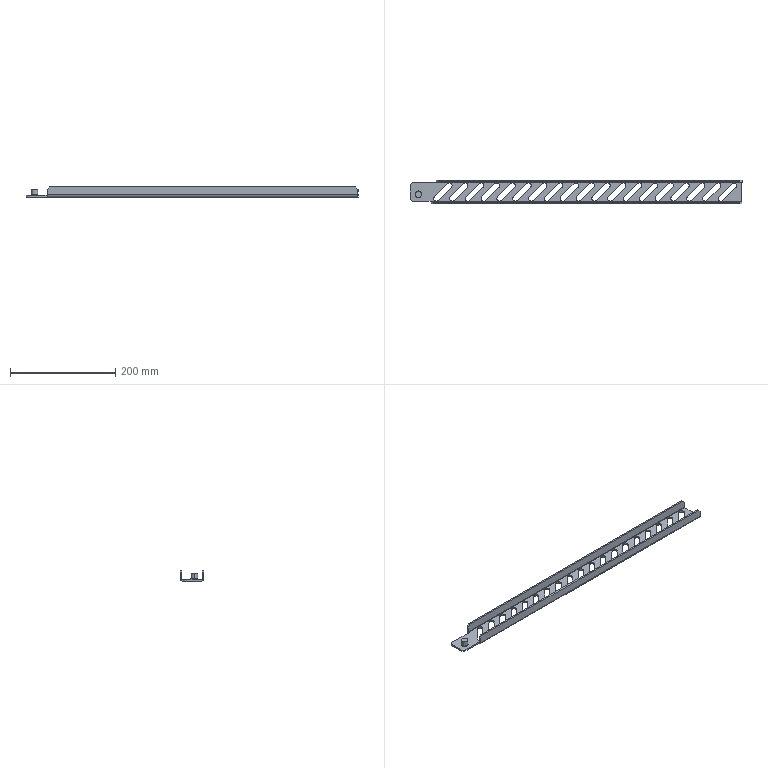Part | SolidWorks | features ICE 3, SM3dBend 2, Chamfer 1, Extrusion 1, FlatPattern 1, LPattern 1, SheetMetal 1, SolidToSheetMetal 1 | 1 solid | 133 faces | box 630 x 45 x 19.073 mm | volume 113043 mm3 | plane 68 | cylinder 65 | commonest cylinder face diameters 10 x57 2 x2 8 x2 12 x2 13 x2